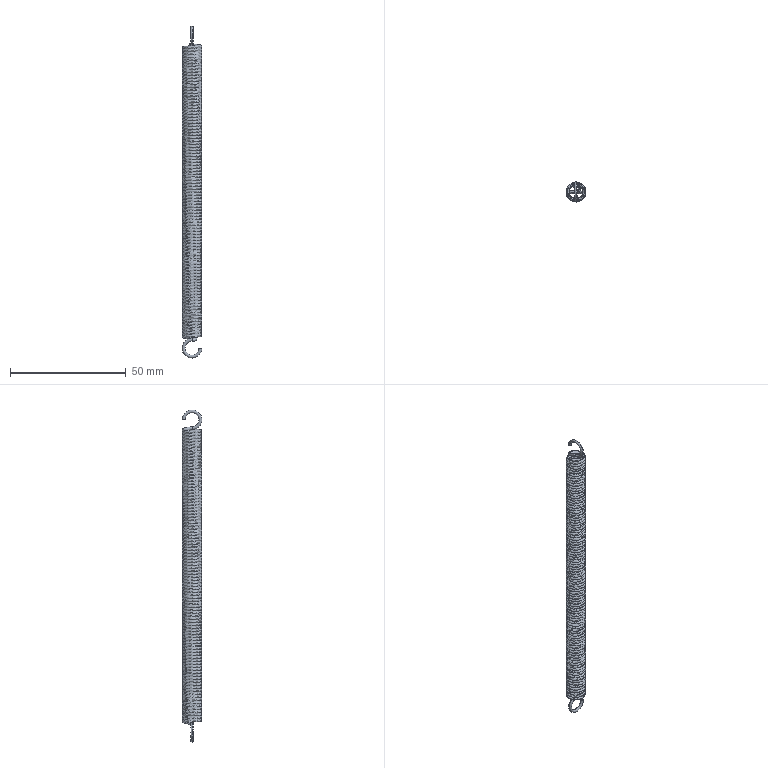Part | SolidWorks | features Sweep 5, 3DProfileFeature 4, Helix 1 | 1 solid | 16 faces | box 8.5 x 8.5 x 143.5 mm | volume 2760 mm3 | spline 6 | plane 6 | torus 4